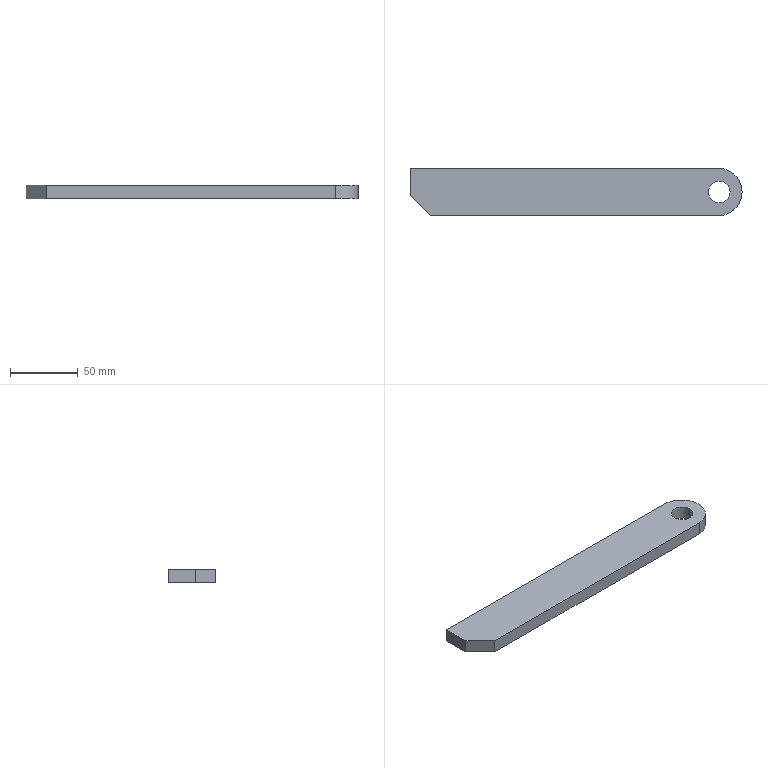Part | SolidWorks | features BaseBody 1 | 1 solid | 10 faces | box 244.844 x 35 x 10 mm | volume 81253 mm3 | plane 6 | cylinder 4 | commonest cylinder face diameters 16 x2 35.082 x2
STEP:
#1=CARTESIAN_POINT('',(212.214,5.017,0.));
#2=VERTEX_POINT('',#1);
#3=CARTESIAN_POINT('',(196.214,5.017,0.));
#4=VERTEX_POINT('',#3);
#5=CARTESIAN_POINT('',(204.214,5.017,0.));
#6=DIRECTION('',(0.,0.,-1.));
#7=DIRECTION('',(1.,0.,0.));
#8=AXIS2_PLACEMENT_3D('',#5,#6,#7);
#9=CIRCLE('',#8,8.);
#10=EDGE_CURVE('',#2,#4,#9,.T.);
#11=ORIENTED_EDGE('',*,*,#10,.T.);
#12=CARTESIAN_POINT('',(196.214,5.017,10.));
#13=VERTEX_POINT('',#12);
#14=CARTESIAN_POINT('',(196.214,5.017,0.));
#15=DIRECTION('',(0.,0.,1.));
#16=VECTOR('',#15,1000.);
#17=LINE('',#14,#16);
#18=EDGE_CURVE('',#4,#13,#17,.T.);
#19=ORIENTED_EDGE('',*,*,#18,.T.);
#20=CARTESIAN_POINT('',(212.214,5.017,10.));
#21=VERTEX_POINT('',#20);
#22=CARTESIAN_POINT('',(204.214,5.017,10.));
#23=DIRECTION('',(0.,0.,-1.));
#24=DIRECTION('',(1.,0.,0.));
#25=AXIS2_PLACEMENT_3D('',#22,#23,#24);
#26=CIRCLE('',#25,8.);
#27=EDGE_CURVE('',#21,#13,#26,.T.);
#28=ORIENTED_EDGE('',*,*,#27,.F.);
#29=CARTESIAN_POINT('',(212.214,5.017,0.));
#30=DIRECTION('',(0.,0.,1.));
#31=VECTOR('',#30,1000.);
#32=LINE('',#29,#31);
#33=EDGE_CURVE('',#2,#21,#32,.T.);
#34=ORIENTED_EDGE('',*,*,#33,.F.);
#35=EDGE_LOOP('',(#11,#19,#28,#34));
#36=FACE_OUTER_BOUND('',#35,.T.);
#37=CARTESIAN_POINT('',(204.214,5.017,0.));
#38=DIRECTION('',(0.,0.,1.));
#39=DIRECTION('',(1.,0.,0.));
#40=AXIS2_PLACEMENT_3D('',#37,#38,#39);
#41=CYLINDRICAL_SURFACE('',#40,8.);
#42=ADVANCED_FACE('',(#36),#41,.F.);
#43=CARTESIAN_POINT('',(204.717,-12.483,0.));
#44=VERTEX_POINT('',#43);
#45=CARTESIAN_POINT('',(221.058,5.017,0.));
#46=VERTEX_POINT('',#45);
#47=CARTESIAN_POINT('',(203.516,5.017,0.));
#48=DIRECTION('',(0.,0.,1.));
#49=DIRECTION('',(1.,0.,0.));
#50=AXIS2_PLACEMENT_3D('',#47,#48,#49);
#51=CIRCLE('',#50,17.541);
#52=EDGE_CURVE('',#44,#46,#51,.T.);
#53=ORIENTED_EDGE('',*,*,#52,.T.);
#54=CARTESIAN_POINT('',(221.058,5.017,10.));
#55=VERTEX_POINT('',#54);
#56=CARTESIAN_POINT('',(221.058,5.017,0.));
#57=DIRECTION('',(0.,0.,1.));
#58=VECTOR('',#57,1000.);
#59=LINE('',#56,#58);
#60=EDGE_CURVE('',#46,#55,#59,.T.);
#61=ORIENTED_EDGE('',*,*,#60,.T.);
#62=CARTESIAN_POINT('',(204.717,-12.483,10.));
#63=VERTEX_POINT('',#62);
#64=CARTESIAN_POINT('',(203.516,5.017,10.));
#65=DIRECTION('',(0.,0.,-1.));
#66=DIRECTION('',(1.,0.,0.));
#67=AXIS2_PLACEMENT_3D('',#64,#65,#66);
#68=CIRCLE('',#67,17.541);
#69=EDGE_CURVE('',#55,#63,#68,.T.);
#70=ORIENTED_EDGE('',*,*,#69,.T.);
#71=CARTESIAN_POINT('',(204.717,-12.483,0.));
#72=DIRECTION('',(0.,0.,-1.));
#73=VECTOR('',#72,1000.);
#74=LINE('',#71,#73);
#75=EDGE_CURVE('',#63,#44,#74,.T.);
#76=ORIENTED_EDGE('',*,*,#75,.T.);
#77=EDGE_LOOP('',(#53,#61,#70,#76));
#78=FACE_OUTER_BOUND('',#77,.T.);
#79=CARTESIAN_POINT('',(203.516,5.017,0.));
#80=DIRECTION('',(0.,0.,1.));
#81=DIRECTION('',(1.,0.,0.));
#82=AXIS2_PLACEMENT_3D('',#79,#80,#81);
#83=CYLINDRICAL_SURFACE('',#82,17.541);
#84=ADVANCED_FACE('',(#78),#83,.T.);
#85=ORIENTED_EDGE('',*,*,#10,.F.);
#86=CARTESIAN_POINT('',(204.214,5.017,0.));
#87=DIRECTION('',(0.,0.,-1.));
#88=DIRECTION('',(1.,0.,0.));
#89=AXIS2_PLACEMENT_3D('',#86,#87,#88);
#90=CIRCLE('',#89,8.);
#91=EDGE_CURVE('',#4,#2,#90,.T.);
#92=ORIENTED_EDGE('',*,*,#91,.F.);
#93=EDGE_LOOP('',(#85,#92));
#94=FACE_BOUND('',#93,.T.);
#95=CARTESIAN_POINT('',(204.717,22.517,0.));
#96=VERTEX_POINT('',#95);
#97=CARTESIAN_POINT('',(-23.786,22.517,0.));
#98=VERTEX_POINT('',#97);
#99=CARTESIAN_POINT('',(97.126,22.517,0.));
#100=DIRECTION('',(-1.,0.,0.));
#101=VECTOR('',#100,1000.);
#102=LINE('',#99,#101);
#103=EDGE_CURVE('',#96,#98,#102,.T.);
#104=ORIENTED_EDGE('',*,*,#103,.F.);
#105=CARTESIAN_POINT('',(203.516,5.017,0.));
#106=DIRECTION('',(0.,0.,1.));
#107=DIRECTION('',(1.,0.,0.));
#108=AXIS2_PLACEMENT_3D('',#105,#106,#107);
#109=CIRCLE('',#108,17.541);
#110=EDGE_CURVE('',#46,#96,#109,.T.);
#111=ORIENTED_EDGE('',*,*,#110,.F.);
#112=ORIENTED_EDGE('',*,*,#52,.F.);
#113=CARTESIAN_POINT('',(-8.786,-12.483,0.));
#114=VERTEX_POINT('',#113);
#115=CARTESIAN_POINT('',(97.126,-12.483,0.));
#116=DIRECTION('',(1.,0.,0.));
#117=VECTOR('',#116,1000.);
#118=LINE('',#115,#117);
#119=EDGE_CURVE('',#114,#44,#118,.T.);
#120=ORIENTED_EDGE('',*,*,#119,.F.);
#121=CARTESIAN_POINT('',(-23.786,2.517,0.));
#122=VERTEX_POINT('',#121);
#123=CARTESIAN_POINT('',(-23.786,2.517,0.));
#124=DIRECTION('',(0.7071,-0.7071,0.));
#125=VECTOR('',#124,1000.);
#126=LINE('',#123,#125);
#127=EDGE_CURVE('',#122,#114,#126,.T.);
#128=ORIENTED_EDGE('',*,*,#127,.F.);
#129=CARTESIAN_POINT('',(-23.786,5.391,0.));
#130=DIRECTION('',(0.,-1.,0.));
#131=VECTOR('',#130,1000.);
#132=LINE('',#129,#131);
#133=EDGE_CURVE('',#98,#122,#132,.T.);
#134=ORIENTED_EDGE('',*,*,#133,.F.);
#135=EDGE_LOOP('',(#104,#111,#112,#120,#128,#134));
#136=FACE_OUTER_BOUND('',#135,.T.);
#137=CARTESIAN_POINT('',(97.126,5.391,0.));
#138=DIRECTION('',(0.,0.,1.));
#139=DIRECTION('',(1.,0.,0.));
#140=AXIS2_PLACEMENT_3D('',#137,#138,#139);
#141=PLANE('',#140);
#142=ADVANCED_FACE('',(#94,#136),#141,.F.);
#143=ORIENTED_EDGE('',*,*,#18,.F.);
#144=ORIENTED_EDGE('',*,*,#91,.T.);
#145=ORIENTED_EDGE('',*,*,#33,.T.);
#146=CARTESIAN_POINT('',(204.214,5.017,10.));
#147=DIRECTION('',(0.,0.,-1.));
#148=DIRECTION('',(1.,0.,0.));
#149=AXIS2_PLACEMENT_3D('',#146,#147,#148);
#150=CIRCLE('',#149,8.);
#151=EDGE_CURVE('',#13,#21,#150,.T.);
#152=ORIENTED_EDGE('',*,*,#151,.F.);
#153=EDGE_LOOP('',(#143,#144,#145,#152));
#154=FACE_OUTER_BOUND('',#153,.T.);
#155=CARTESIAN_POINT('',(204.214,5.017,0.));
#156=DIRECTION('',(0.,0.,1.));
#157=DIRECTION('',(1.,0.,0.));
#158=AXIS2_PLACEMENT_3D('',#155,#156,#157);
#159=CYLINDRICAL_SURFACE('',#158,8.);
#160=ADVANCED_FACE('',(#154),#159,.F.);
#161=ORIENTED_EDGE('',*,*,#133,.T.);
#162=CARTESIAN_POINT('',(-23.786,2.517,10.));
#163=VERTEX_POINT('',#162);
#164=CARTESIAN_POINT('',(-23.786,2.517,0.));
#165=DIRECTION('',(0.,0.,1.));
#166=VECTOR('',#165,1000.);
#167=LINE('',#164,#166);
#168=EDGE_CURVE('',#122,#163,#167,.T.);
#169=ORIENTED_EDGE('',*,*,#168,.T.);
#170=CARTESIAN_POINT('',(-23.786,22.517,10.));
#171=VERTEX_POINT('',#170);
#172=CARTESIAN_POINT('',(-23.786,2.517,10.));
#173=DIRECTION('',(0.,1.,0.));
#174=VECTOR('',#173,1000.);
#175=LINE('',#172,#174);
#176=EDGE_CURVE('',#163,#171,#175,.T.);
#177=ORIENTED_EDGE('',*,*,#176,.T.);
#178=CARTESIAN_POINT('',(-23.786,22.517,0.));
#179=DIRECTION('',(0.,0.,-1.));
#180=VECTOR('',#179,1000.);
#181=LINE('',#178,#180);
#182=EDGE_CURVE('',#171,#98,#181,.T.);
#183=ORIENTED_EDGE('',*,*,#182,.T.);
#184=EDGE_LOOP('',(#161,#169,#177,#183));
#185=FACE_OUTER_BOUND('',#184,.T.);
#186=CARTESIAN_POINT('',(-23.786,2.517,0.));
#187=DIRECTION('',(-1.,0.,0.));
#188=DIRECTION('',(0.,-1.,0.));
#189=AXIS2_PLACEMENT_3D('',#186,#187,#188);
#190=PLANE('',#189);
#191=ADVANCED_FACE('',(#185),#190,.T.);
#192=ORIENTED_EDGE('',*,*,#103,.T.);
#193=ORIENTED_EDGE('',*,*,#182,.F.);
#194=CARTESIAN_POINT('',(204.717,22.517,10.));
#195=VERTEX_POINT('',#194);
#196=CARTESIAN_POINT('',(202.316,22.517,10.));
#197=DIRECTION('',(1.,0.,0.));
#198=VECTOR('',#197,1000.);
#199=LINE('',#196,#198);
#200=EDGE_CURVE('',#171,#195,#199,.T.);
#201=ORIENTED_EDGE('',*,*,#200,.T.);
#202=CARTESIAN_POINT('',(204.717,22.517,0.));
#203=DIRECTION('',(0.,0.,-1.));
#204=VECTOR('',#203,1000.);
#205=LINE('',#202,#204);
#206=EDGE_CURVE('',#195,#96,#205,.T.);
#207=ORIENTED_EDGE('',*,*,#206,.T.);
#208=EDGE_LOOP('',(#192,#193,#201,#207));
#209=FACE_OUTER_BOUND('',#208,.T.);
#210=CARTESIAN_POINT('',(202.316,22.517,0.));
#211=DIRECTION('',(0.,1.,0.));
#212=DIRECTION('',(0.,0.,1.));
#213=AXIS2_PLACEMENT_3D('',#210,#211,#212);
#214=PLANE('',#213);
#215=ADVANCED_FACE('',(#209),#214,.T.);
#216=ORIENTED_EDGE('',*,*,#60,.F.);
#217=ORIENTED_EDGE('',*,*,#110,.T.);
#218=ORIENTED_EDGE('',*,*,#206,.F.);
#219=CARTESIAN_POINT('',(203.516,5.017,10.));
#220=DIRECTION('',(0.,0.,-1.));
#221=DIRECTION('',(1.,0.,0.));
#222=AXIS2_PLACEMENT_3D('',#219,#220,#221);
#223=CIRCLE('',#222,17.541);
#224=EDGE_CURVE('',#195,#55,#223,.T.);
#225=ORIENTED_EDGE('',*,*,#224,.T.);
#226=EDGE_LOOP('',(#216,#217,#218,#225));
#227=FACE_OUTER_BOUND('',#226,.T.);
#228=CARTESIAN_POINT('',(203.516,5.017,0.));
#229=DIRECTION('',(0.,0.,1.));
#230=DIRECTION('',(1.,0.,0.));
#231=AXIS2_PLACEMENT_3D('',#228,#229,#230);
#232=CYLINDRICAL_SURFACE('',#231,17.541);
#233=ADVANCED_FACE('',(#227),#232,.T.);
#234=ORIENTED_EDGE('',*,*,#119,.T.);
#235=ORIENTED_EDGE('',*,*,#75,.F.);
#236=CARTESIAN_POINT('',(-8.786,-12.483,10.));
#237=VERTEX_POINT('',#236);
#238=CARTESIAN_POINT('',(202.316,-12.483,10.));
#239=DIRECTION('',(-1.,0.,0.));
#240=VECTOR('',#239,1000.);
#241=LINE('',#238,#240);
#242=EDGE_CURVE('',#63,#237,#241,.T.);
#243=ORIENTED_EDGE('',*,*,#242,.T.);
#244=CARTESIAN_POINT('',(-8.786,-12.483,0.));
#245=DIRECTION('',(0.,0.,-1.));
#246=VECTOR('',#245,1000.);
#247=LINE('',#244,#246);
#248=EDGE_CURVE('',#237,#114,#247,.T.);
#249=ORIENTED_EDGE('',*,*,#248,.T.);
#250=EDGE_LOOP('',(#234,#235,#243,#249));
#251=FACE_OUTER_BOUND('',#250,.T.);
#252=CARTESIAN_POINT('',(202.316,-12.483,0.));
#253=DIRECTION('',(0.,-1.,0.));
#254=DIRECTION('',(1.,0.,0.));
#255=AXIS2_PLACEMENT_3D('',#252,#253,#254);
#256=PLANE('',#255);
#257=ADVANCED_FACE('',(#251),#256,.T.);
#258=ORIENTED_EDGE('',*,*,#127,.T.);
#259=ORIENTED_EDGE('',*,*,#248,.F.);
#260=CARTESIAN_POINT('',(-8.786,-12.483,10.));
#261=DIRECTION('',(-0.7071,0.7071,0.));
#262=VECTOR('',#261,1000.);
#263=LINE('',#260,#262);
#264=EDGE_CURVE('',#237,#163,#263,.T.);
#265=ORIENTED_EDGE('',*,*,#264,.T.);
#266=ORIENTED_EDGE('',*,*,#168,.F.);
#267=EDGE_LOOP('',(#258,#259,#265,#266));
#268=FACE_OUTER_BOUND('',#267,.T.);
#269=CARTESIAN_POINT('',(-8.786,-12.483,0.));
#270=DIRECTION('',(-0.7071,-0.7071,0.));
#271=DIRECTION('',(0.7071,-0.7071,0.));
#272=AXIS2_PLACEMENT_3D('',#269,#270,#271);
#273=PLANE('',#272);
#274=ADVANCED_FACE('',(#268),#273,.T.);
#275=ORIENTED_EDGE('',*,*,#27,.T.);
#276=ORIENTED_EDGE('',*,*,#151,.T.);
#277=EDGE_LOOP('',(#275,#276));
#278=FACE_BOUND('',#277,.T.);
#279=ORIENTED_EDGE('',*,*,#242,.F.);
#280=ORIENTED_EDGE('',*,*,#69,.F.);
#281=ORIENTED_EDGE('',*,*,#224,.F.);
#282=ORIENTED_EDGE('',*,*,#200,.F.);
#283=ORIENTED_EDGE('',*,*,#176,.F.);
#284=ORIENTED_EDGE('',*,*,#264,.F.);
#285=EDGE_LOOP('',(#279,#280,#281,#282,#283,#284));
#286=FACE_OUTER_BOUND('',#285,.T.);
#287=CARTESIAN_POINT('',(97.126,5.391,10.));
#288=DIRECTION('',(0.,0.,1.));
#289=DIRECTION('',(1.,0.,0.));
#290=AXIS2_PLACEMENT_3D('',#287,#288,#289);
#291=PLANE('',#290);
#292=ADVANCED_FACE('',(#278,#286),#291,.T.);
#293=CLOSED_SHELL('',(#42,#84,#142,#160,#191,#215,#233,#257,#274,#292));
#294=MANIFOLD_SOLID_BREP('',#293);
#295=CARTESIAN_POINT('',(0.,0.,0.));
#296=DIRECTION('',(0.,0.,1.));
#297=DIRECTION('',(1.,0.,0.));
#298=AXIS2_PLACEMENT_3D('',#295,#296,#297);
#299=(LENGTH_UNIT()NAMED_UNIT(*)SI_UNIT(.MILLI.,.METRE.));
#300=UNCERTAINTY_MEASURE_WITH_UNIT(LENGTH_MEASURE(0.00001),#299,'','');
#301=(NAMED_UNIT(*)PLANE_ANGLE_UNIT()SI_UNIT($,.RADIAN.));
#302=(NAMED_UNIT(*)SI_UNIT($,.STERADIAN.)SOLID_ANGLE_UNIT());
#303=(GEOMETRIC_REPRESENTATION_CONTEXT(3)GLOBAL_UNCERTAINTY_ASSIGNED_CONTEXT((#300))GLOBAL_UNIT_ASSIGNED_CONTEXT((#299,#301,#302))REPRESENTATION_CONTEXT('',''));
#304=ADVANCED_BREP_SHAPE_REPRESENTATION('',(#294,#298),#303);